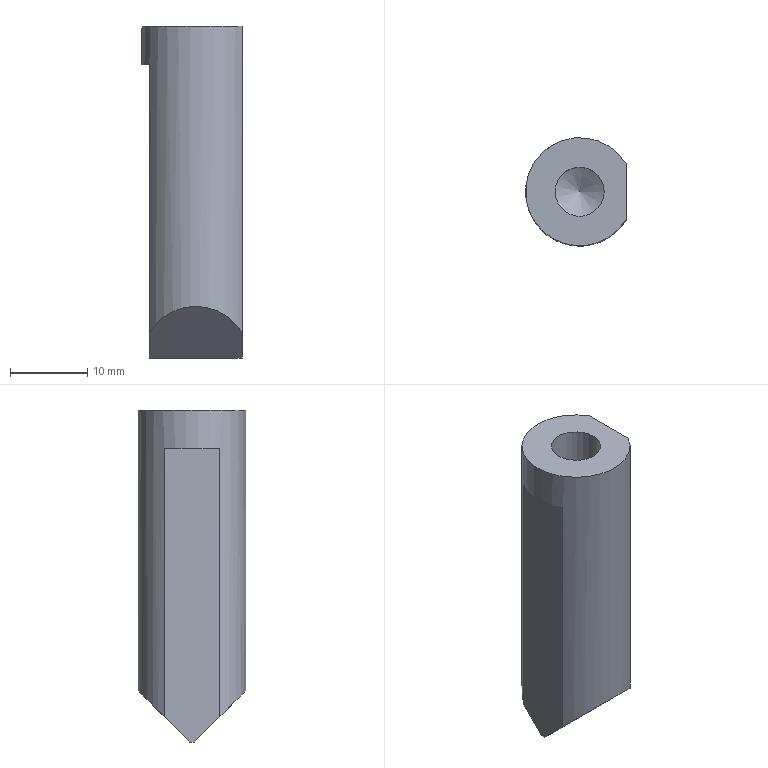Part | STEP file | 1_id278_x_t | 1 solid | 10 faces | box 13 x 14 x 43 mm | volume 5330 mm3 | plane 7 | cylinder 2 | cone 1 | commonest cylinder face diameters 6.35 x1 14 x1
STEP:
#1=CARTESIAN_POINT('',(0.,0.,0.));
#2=DIRECTION('',(0.,0.,1.));
#3=DIRECTION('',(1.,0.,0.));
#4=AXIS2_PLACEMENT_3D('',#1,#2,#3);
#5=CARTESIAN_POINT('',(759.425,181.106,-65.394));
#6=VERTEX_POINT('',#5);
#7=CARTESIAN_POINT('',(759.425,177.82,-68.68));
#8=VERTEX_POINT('',#7);
#9=CARTESIAN_POINT('',(759.425,178.5,-68.));
#10=DIRECTION('',(0.,-0.7071,-0.7071));
#11=VECTOR('',#10,1.);
#12=LINE('',#9,#11);
#13=CARTESIAN_POINT('',(771.425,178.5,-68.));
#14=DIRECTION('',(0.,-0.7071,0.7071));
#15=DIRECTION('',(0.,0.7071,0.7071));
#16=AXIS2_PLACEMENT_3D('',#13,#14,#15);
#17=PLANE('',#16);
#18=CARTESIAN_POINT('',(0.,12.));
#19=DIRECTION('',(-1.,0.));
#20=VECTOR('',#19,1.);
#21=LINE('',#18,#20);
#22=(GEOMETRIC_REPRESENTATION_CONTEXT(2)PARAMETRIC_REPRESENTATION_CONTEXT()REPRESENTATION_CONTEXT('',''));
#23=DEFINITIONAL_REPRESENTATION('',(#21),#22);
#24=PCURVE('',#17,#23);
#25=CARTESIAN_POINT('',(759.425,168.899,-15.68));
#26=DIRECTION('',(1.,0.,0.));
#27=DIRECTION('',(0.,0.,-1.));
#28=AXIS2_PLACEMENT_3D('',#25,#26,#27);
#29=PLANE('',#28);
#30=CARTESIAN_POINT('',(52.32,9.601));
#31=DIRECTION('',(0.7071,-0.7071));
#32=VECTOR('',#31,1.);
#33=LINE('',#30,#32);
#34=(GEOMETRIC_REPRESENTATION_CONTEXT(2)PARAMETRIC_REPRESENTATION_CONTEXT()REPRESENTATION_CONTEXT('',''));
#35=DEFINITIONAL_REPRESENTATION('',(#33),#34);
#36=PCURVE('',#29,#35);
#37=SURFACE_CURVE('',#12,(#24,#36),.PCURVE_S1.);
#38=EDGE_CURVE('',#6,#8,#37,.T.);
#39=ORIENTED_EDGE('',*,*,#38,.F.);
#40=CARTESIAN_POINT('',(771.425,181.106,-65.394));
#41=VERTEX_POINT('',#40);
#42=CARTESIAN_POINT('',(765.425,177.5,-69.));
#43=DIRECTION('',(0.,-0.7071,0.7071));
#44=DIRECTION('',(0.,-0.7071,-0.7071));
#45=AXIS2_PLACEMENT_3D('',#42,#43,#44);
#46=ELLIPSE('',#45,9.899,7.);
#47=CARTESIAN_POINT('',(-1.414,6.));
#48=DIRECTION('',(-1.,0.));
#49=AXIS2_PLACEMENT_2D('',#47,#48);
#50=ELLIPSE('',#49,9.899,7.);
#51=(GEOMETRIC_REPRESENTATION_CONTEXT(2)PARAMETRIC_REPRESENTATION_CONTEXT()REPRESENTATION_CONTEXT('',''));
#52=DEFINITIONAL_REPRESENTATION('',(#50),#51);
#53=PCURVE('',#17,#52);
#54=CARTESIAN_POINT('',(765.425,177.5,17.));
#55=DIRECTION('',(0.,0.,-1.));
#56=DIRECTION('',(0.,1.,0.));
#57=AXIS2_PLACEMENT_3D('',#54,#55,#56);
#58=CYLINDRICAL_SURFACE('',#57,7.);
#59=CARTESIAN_POINT('',(7.313,82.394));
#60=CARTESIAN_POINT('',(7.282,82.207));
#61=CARTESIAN_POINT('',(7.219,81.843));
#62=CARTESIAN_POINT('',(7.126,81.334));
#63=CARTESIAN_POINT('',(7.032,80.865));
#64=CARTESIAN_POINT('',(6.938,80.442));
#65=CARTESIAN_POINT('',(6.845,80.067));
#66=CARTESIAN_POINT('',(6.751,79.744));
#67=CARTESIAN_POINT('',(6.658,79.475));
#68=CARTESIAN_POINT('',(6.564,79.264));
#69=CARTESIAN_POINT('',(6.47,79.112));
#70=CARTESIAN_POINT('',(6.377,79.02));
#71=CARTESIAN_POINT('',(6.283,78.99));
#72=CARTESIAN_POINT('',(6.19,79.02));
#73=CARTESIAN_POINT('',(6.096,79.112));
#74=CARTESIAN_POINT('',(6.002,79.264));
#75=CARTESIAN_POINT('',(5.909,79.475));
#76=CARTESIAN_POINT('',(5.815,79.744));
#77=CARTESIAN_POINT('',(5.722,80.067));
#78=CARTESIAN_POINT('',(5.628,80.442));
#79=CARTESIAN_POINT('',(5.534,80.865));
#80=CARTESIAN_POINT('',(5.441,81.334));
#81=CARTESIAN_POINT('',(5.347,81.843));
#82=CARTESIAN_POINT('',(5.285,82.207));
#83=CARTESIAN_POINT('',(5.253,82.394));
#84=B_SPLINE_CURVE_WITH_KNOTS('',3,(#59,#60,#61,#62,#63,#64,#65,#66,#67,#68,#69,#70,#71,#72,#73,#74,#75,#76,#77,#78,#79,#80,#81,#82,#83),.UNSPECIFIED.,.F.,.F.,(4,1,1,1,1,1,1,1,1,1,1,1,1,1,1,1,1,1,1,1,1,1,4),(2.112,2.206,2.299,2.393,2.486,2.58,2.674,2.767,2.861,2.954,3.048,3.142,3.235,3.329,3.422,3.516,3.61,3.703,3.797,3.89,3.984,4.078,4.171),.QUASI_UNIFORM_KNOTS.);
#85=(GEOMETRIC_REPRESENTATION_CONTEXT(2)PARAMETRIC_REPRESENTATION_CONTEXT()REPRESENTATION_CONTEXT('',''));
#86=DEFINITIONAL_REPRESENTATION('',(#84),#85);
#87=PCURVE('',#58,#86);
#88=SURFACE_CURVE('',#46,(#53,#87),.PCURVE_S1.);
#89=EDGE_CURVE('',#41,#6,#88,.T.);
#90=ORIENTED_EDGE('',*,*,#89,.F.);
#91=CARTESIAN_POINT('',(771.425,177.82,-68.68));
#92=VERTEX_POINT('',#91);
#93=CARTESIAN_POINT('',(771.425,178.5,-68.));
#94=DIRECTION('',(0.,0.7071,0.7071));
#95=VECTOR('',#94,1.);
#96=LINE('',#93,#95);
#97=CARTESIAN_POINT('',(0.,0.));
#98=DIRECTION('',(1.,0.));
#99=VECTOR('',#98,1.);
#100=LINE('',#97,#99);
#101=(GEOMETRIC_REPRESENTATION_CONTEXT(2)PARAMETRIC_REPRESENTATION_CONTEXT()REPRESENTATION_CONTEXT('',''));
#102=DEFINITIONAL_REPRESENTATION('',(#100),#101);
#103=PCURVE('',#17,#102);
#104=CARTESIAN_POINT('',(771.425,170.46,30.));
#105=DIRECTION('',(1.,0.,0.));
#106=DIRECTION('',(0.,0.,1.));
#107=AXIS2_PLACEMENT_3D('',#104,#105,#106);
#108=PLANE('',#107);
#109=CARTESIAN_POINT('',(-98.,-8.04));
#110=DIRECTION('',(0.7071,-0.7071));
#111=VECTOR('',#110,1.);
#112=LINE('',#109,#111);
#113=(GEOMETRIC_REPRESENTATION_CONTEXT(2)PARAMETRIC_REPRESENTATION_CONTEXT()REPRESENTATION_CONTEXT('',''));
#114=DEFINITIONAL_REPRESENTATION('',(#112),#113);
#115=PCURVE('',#108,#114);
#116=SURFACE_CURVE('',#96,(#103,#115),.PCURVE_S1.);
#117=EDGE_CURVE('',#92,#41,#116,.T.);
#118=ORIENTED_EDGE('',*,*,#117,.F.);
#119=CARTESIAN_POINT('',(771.425,177.82,-68.68));
#120=DIRECTION('',(-1.,0.,0.));
#121=VECTOR('',#120,1.);
#122=LINE('',#119,#121);
#123=CARTESIAN_POINT('',(-0.9617,0.));
#124=DIRECTION('',(0.,1.));
#125=VECTOR('',#124,1.);
#126=LINE('',#123,#125);
#127=(GEOMETRIC_REPRESENTATION_CONTEXT(2)PARAMETRIC_REPRESENTATION_CONTEXT()REPRESENTATION_CONTEXT('',''));
#128=DEFINITIONAL_REPRESENTATION('',(#126),#127);
#129=PCURVE('',#17,#128);
#130=CARTESIAN_POINT('',(765.425,177.5,-68.68));
#131=DIRECTION('',(0.,0.,-1.));
#132=DIRECTION('',(0.,1.,0.));
#133=AXIS2_PLACEMENT_3D('',#130,#131,#132);
#134=PLANE('',#133);
#135=CARTESIAN_POINT('',(0.32,6.));
#136=DIRECTION('',(0.,-1.));
#137=VECTOR('',#136,1.);
#138=LINE('',#135,#137);
#139=(GEOMETRIC_REPRESENTATION_CONTEXT(2)PARAMETRIC_REPRESENTATION_CONTEXT()REPRESENTATION_CONTEXT('',''));
#140=DEFINITIONAL_REPRESENTATION('',(#138),#139);
#141=PCURVE('',#134,#140);
#142=SURFACE_CURVE('',#122,(#129,#141),.PCURVE_S1.);
#143=EDGE_CURVE('',#92,#8,#142,.T.);
#144=ORIENTED_EDGE('',*,*,#143,.T.);
#145=EDGE_LOOP('',(#39,#90,#118,#144));
#146=FACE_BOUND('',#145,.T.);
#147=ADVANCED_FACE('',(#146),#17,.F.);
#148=CARTESIAN_POINT('',(759.425,177.18,-68.68));
#149=VERTEX_POINT('',#148);
#150=CARTESIAN_POINT('',(759.425,177.5,-68.68));
#151=DIRECTION('',(0.,-1.,0.));
#152=VECTOR('',#151,1.);
#153=LINE('',#150,#152);
#154=CARTESIAN_POINT('',(0.,-6.));
#155=DIRECTION('',(-1.,0.));
#156=VECTOR('',#155,1.);
#157=LINE('',#154,#156);
#158=(GEOMETRIC_REPRESENTATION_CONTEXT(2)PARAMETRIC_REPRESENTATION_CONTEXT()REPRESENTATION_CONTEXT('',''));
#159=DEFINITIONAL_REPRESENTATION('',(#157),#158);
#160=PCURVE('',#134,#159);
#161=CARTESIAN_POINT('',(53.,8.601));
#162=DIRECTION('',(0.,-1.));
#163=VECTOR('',#162,1.);
#164=LINE('',#161,#163);
#165=(GEOMETRIC_REPRESENTATION_CONTEXT(2)PARAMETRIC_REPRESENTATION_CONTEXT()REPRESENTATION_CONTEXT('',''));
#166=DEFINITIONAL_REPRESENTATION('',(#164),#165);
#167=PCURVE('',#29,#166);
#168=SURFACE_CURVE('',#153,(#160,#167),.PCURVE_S1.);
#169=EDGE_CURVE('',#8,#149,#168,.T.);
#170=ORIENTED_EDGE('',*,*,#169,.F.);
#171=ORIENTED_EDGE('',*,*,#143,.F.);
#172=CARTESIAN_POINT('',(771.425,177.18,-68.68));
#173=VERTEX_POINT('',#172);
#174=CARTESIAN_POINT('',(771.425,170.46,-68.68));
#175=DIRECTION('',(0.,1.,0.));
#176=VECTOR('',#175,1.);
#177=LINE('',#174,#176);
#178=CARTESIAN_POINT('',(-7.04,6.));
#179=DIRECTION('',(1.,0.));
#180=VECTOR('',#179,1.);
#181=LINE('',#178,#180);
#182=(GEOMETRIC_REPRESENTATION_CONTEXT(2)PARAMETRIC_REPRESENTATION_CONTEXT()REPRESENTATION_CONTEXT('',''));
#183=DEFINITIONAL_REPRESENTATION('',(#181),#182);
#184=PCURVE('',#134,#183);
#185=CARTESIAN_POINT('',(-98.68,0.));
#186=DIRECTION('',(0.,-1.));
#187=VECTOR('',#186,1.);
#188=LINE('',#185,#187);
#189=(GEOMETRIC_REPRESENTATION_CONTEXT(2)PARAMETRIC_REPRESENTATION_CONTEXT()REPRESENTATION_CONTEXT('',''));
#190=DEFINITIONAL_REPRESENTATION('',(#188),#189);
#191=PCURVE('',#108,#190);
#192=SURFACE_CURVE('',#177,(#184,#191),.PCURVE_S1.);
#193=EDGE_CURVE('',#173,#92,#192,.T.);
#194=ORIENTED_EDGE('',*,*,#193,.F.);
#195=CARTESIAN_POINT('',(765.425,177.18,-68.68));
#196=DIRECTION('',(-1.,0.,0.));
#197=VECTOR('',#196,1.);
#198=LINE('',#195,#197);
#199=CARTESIAN_POINT('',(-0.32,0.));
#200=DIRECTION('',(0.,-1.));
#201=VECTOR('',#200,1.);
#202=LINE('',#199,#201);
#203=(GEOMETRIC_REPRESENTATION_CONTEXT(2)PARAMETRIC_REPRESENTATION_CONTEXT()REPRESENTATION_CONTEXT('',''));
#204=DEFINITIONAL_REPRESENTATION('',(#202),#203);
#205=PCURVE('',#134,#204);
#206=CARTESIAN_POINT('',(771.425,176.5,-68.));
#207=DIRECTION('',(0.,0.7071,0.7071));
#208=DIRECTION('',(0.,-0.7071,0.7071));
#209=AXIS2_PLACEMENT_3D('',#206,#207,#208);
#210=PLANE('',#209);
#211=CARTESIAN_POINT('',(-0.9617,-6.));
#212=DIRECTION('',(0.,-1.));
#213=VECTOR('',#212,1.);
#214=LINE('',#211,#213);
#215=(GEOMETRIC_REPRESENTATION_CONTEXT(2)PARAMETRIC_REPRESENTATION_CONTEXT()REPRESENTATION_CONTEXT('',''));
#216=DEFINITIONAL_REPRESENTATION('',(#214),#215);
#217=PCURVE('',#210,#216);
#218=SURFACE_CURVE('',#198,(#205,#217),.PCURVE_S1.);
#219=EDGE_CURVE('',#173,#149,#218,.T.);
#220=ORIENTED_EDGE('',*,*,#219,.T.);
#221=EDGE_LOOP('',(#170,#171,#194,#220));
#222=FACE_BOUND('',#221,.T.);
#223=ADVANCED_FACE('',(#222),#134,.T.);
#224=CARTESIAN_POINT('',(759.425,173.894,-65.394));
#225=VERTEX_POINT('',#224);
#226=CARTESIAN_POINT('',(759.425,176.5,-68.));
#227=DIRECTION('',(0.,-0.7071,0.7071));
#228=VECTOR('',#227,1.);
#229=LINE('',#226,#228);
#230=CARTESIAN_POINT('',(0.,-12.));
#231=DIRECTION('',(1.,0.));
#232=VECTOR('',#231,1.);
#233=LINE('',#230,#232);
#234=(GEOMETRIC_REPRESENTATION_CONTEXT(2)PARAMETRIC_REPRESENTATION_CONTEXT()REPRESENTATION_CONTEXT('',''));
#235=DEFINITIONAL_REPRESENTATION('',(#233),#234);
#236=PCURVE('',#210,#235);
#237=CARTESIAN_POINT('',(52.32,7.601));
#238=DIRECTION('',(-0.7071,-0.7071));
#239=VECTOR('',#238,1.);
#240=LINE('',#237,#239);
#241=(GEOMETRIC_REPRESENTATION_CONTEXT(2)PARAMETRIC_REPRESENTATION_CONTEXT()REPRESENTATION_CONTEXT('',''));
#242=DEFINITIONAL_REPRESENTATION('',(#240),#241);
#243=PCURVE('',#29,#242);
#244=SURFACE_CURVE('',#229,(#236,#243),.PCURVE_S1.);
#245=EDGE_CURVE('',#149,#225,#244,.T.);
#246=ORIENTED_EDGE('',*,*,#245,.F.);
#247=ORIENTED_EDGE('',*,*,#219,.F.);
#248=CARTESIAN_POINT('',(771.425,173.894,-65.394));
#249=VERTEX_POINT('',#248);
#250=CARTESIAN_POINT('',(771.425,176.5,-68.));
#251=DIRECTION('',(0.,-0.7071,0.7071));
#252=VECTOR('',#251,1.);
#253=LINE('',#250,#252);
#254=CARTESIAN_POINT('',(0.,0.));
#255=DIRECTION('',(1.,0.));
#256=VECTOR('',#255,1.);
#257=LINE('',#254,#256);
#258=(GEOMETRIC_REPRESENTATION_CONTEXT(2)PARAMETRIC_REPRESENTATION_CONTEXT()REPRESENTATION_CONTEXT('',''));
#259=DEFINITIONAL_REPRESENTATION('',(#257),#258);
#260=PCURVE('',#210,#259);
#261=CARTESIAN_POINT('',(-98.,-6.04));
#262=DIRECTION('',(0.7071,0.7071));
#263=VECTOR('',#262,1.);
#264=LINE('',#261,#263);
#265=(GEOMETRIC_REPRESENTATION_CONTEXT(2)PARAMETRIC_REPRESENTATION_CONTEXT()REPRESENTATION_CONTEXT('',''));
#266=DEFINITIONAL_REPRESENTATION('',(#264),#265);
#267=PCURVE('',#108,#266);
#268=SURFACE_CURVE('',#253,(#260,#267),.PCURVE_S1.);
#269=EDGE_CURVE('',#173,#249,#268,.T.);
#270=ORIENTED_EDGE('',*,*,#269,.T.);
#271=CARTESIAN_POINT('',(765.425,177.5,-69.));
#272=DIRECTION('',(0.,0.7071,0.7071));
#273=DIRECTION('',(0.,0.7071,-0.7071));
#274=AXIS2_PLACEMENT_3D('',#271,#272,#273);
#275=ELLIPSE('',#274,9.899,7.);
#276=CARTESIAN_POINT('',(-1.414,-6.));
#277=DIRECTION('',(-1.,0.));
#278=AXIS2_PLACEMENT_2D('',#276,#277);
#279=ELLIPSE('',#278,9.899,7.);
#280=(GEOMETRIC_REPRESENTATION_CONTEXT(2)PARAMETRIC_REPRESENTATION_CONTEXT()REPRESENTATION_CONTEXT('',''));
#281=DEFINITIONAL_REPRESENTATION('',(#279),#280);
#282=PCURVE('',#210,#281);
#283=CARTESIAN_POINT('',(4.171,82.394));
#284=CARTESIAN_POINT('',(4.14,82.207));
#285=CARTESIAN_POINT('',(4.078,81.843));
#286=CARTESIAN_POINT('',(3.984,81.334));
#287=CARTESIAN_POINT('',(3.89,80.865));
#288=CARTESIAN_POINT('',(3.797,80.442));
#289=CARTESIAN_POINT('',(3.703,80.067));
#290=CARTESIAN_POINT('',(3.61,79.744));
#291=CARTESIAN_POINT('',(3.516,79.475));
#292=CARTESIAN_POINT('',(3.422,79.264));
#293=CARTESIAN_POINT('',(3.329,79.112));
#294=CARTESIAN_POINT('',(3.235,79.02));
#295=CARTESIAN_POINT('',(3.142,78.99));
#296=CARTESIAN_POINT('',(3.048,79.02));
#297=CARTESIAN_POINT('',(2.954,79.112));
#298=CARTESIAN_POINT('',(2.861,79.264));
#299=CARTESIAN_POINT('',(2.767,79.475));
#300=CARTESIAN_POINT('',(2.674,79.744));
#301=CARTESIAN_POINT('',(2.58,80.067));
#302=CARTESIAN_POINT('',(2.486,80.442));
#303=CARTESIAN_POINT('',(2.393,80.865));
#304=CARTESIAN_POINT('',(2.299,81.334));
#305=CARTESIAN_POINT('',(2.206,81.843));
#306=CARTESIAN_POINT('',(2.143,82.207));
#307=CARTESIAN_POINT('',(2.112,82.394));
#308=B_SPLINE_CURVE_WITH_KNOTS('',3,(#283,#284,#285,#286,#287,#288,#289,#290,#291,#292,#293,#294,#295,#296,#297,#298,#299,#300,#301,#302,#303,#304,#305,#306,#307),.UNSPECIFIED.,.F.,.F.,(4,1,1,1,1,1,1,1,1,1,1,1,1,1,1,1,1,1,1,1,1,1,4),(2.112,2.206,2.299,2.393,2.486,2.58,2.674,2.767,2.861,2.954,3.048,3.142,3.235,3.329,3.422,3.516,3.61,3.703,3.797,3.89,3.984,4.078,4.171),.QUASI_UNIFORM_KNOTS.);
#309=(GEOMETRIC_REPRESENTATION_CONTEXT(2)PARAMETRIC_REPRESENTATION_CONTEXT()REPRESENTATION_CONTEXT('',''));
#310=DEFINITIONAL_REPRESENTATION('',(#308),#309);
#311=PCURVE('',#58,#310);
#312=SURFACE_CURVE('',#275,(#282,#311),.PCURVE_S1.);
#313=EDGE_CURVE('',#225,#249,#312,.T.);
#314=ORIENTED_EDGE('',*,*,#313,.F.);
#315=EDGE_LOOP('',(#246,#247,#270,#314));
#316=FACE_BOUND('',#315,.T.);
#317=ADVANCED_FACE('',(#316),#210,.F.);
#318=CARTESIAN_POINT('',(771.425,181.106,-25.68));
#319=VERTEX_POINT('',#318);
#320=CARTESIAN_POINT('',(771.425,181.106,17.));
#321=DIRECTION('',(0.,0.,-1.));
#322=VECTOR('',#321,1.);
#323=LINE('',#320,#322);
#324=CARTESIAN_POINT('',(-13.,-10.645));
#325=DIRECTION('',(-1.,0.));
#326=VECTOR('',#325,1.);
#327=LINE('',#324,#326);
#328=(GEOMETRIC_REPRESENTATION_CONTEXT(2)PARAMETRIC_REPRESENTATION_CONTEXT()REPRESENTATION_CONTEXT('',''));
#329=DEFINITIONAL_REPRESENTATION('',(#327),#328);
#330=PCURVE('',#108,#329);
#331=CARTESIAN_POINT('',(7.313,0.));
#332=DIRECTION('',(0.,1.));
#333=VECTOR('',#332,1.);
#334=LINE('',#331,#333);
#335=(GEOMETRIC_REPRESENTATION_CONTEXT(2)PARAMETRIC_REPRESENTATION_CONTEXT()REPRESENTATION_CONTEXT('',''));
#336=DEFINITIONAL_REPRESENTATION('',(#334),#335);
#337=PCURVE('',#58,#336);
#338=SURFACE_CURVE('',#323,(#330,#337),.PCURVE_S1.);
#339=EDGE_CURVE('',#319,#41,#338,.T.);
#340=ORIENTED_EDGE('',*,*,#339,.F.);
#341=CARTESIAN_POINT('',(771.425,173.894,-25.68));
#342=VERTEX_POINT('',#341);
#343=CARTESIAN_POINT('',(771.425,177.5,-25.68));
#344=DIRECTION('',(0.,-1.,0.));
#345=VECTOR('',#344,1.);
#346=LINE('',#343,#345);
#347=CARTESIAN_POINT('',(-55.68,-7.04));
#348=DIRECTION('',(0.,1.));
#349=VECTOR('',#348,1.);
#350=LINE('',#347,#349);
#351=(GEOMETRIC_REPRESENTATION_CONTEXT(2)PARAMETRIC_REPRESENTATION_CONTEXT()REPRESENTATION_CONTEXT('',''));
#352=DEFINITIONAL_REPRESENTATION('',(#350),#351);
#353=PCURVE('',#108,#352);
#354=CARTESIAN_POINT('',(780.775,177.5,-25.68));
#355=DIRECTION('',(0.,0.,-1.));
#356=DIRECTION('',(0.,1.,0.));
#357=AXIS2_PLACEMENT_3D('',#354,#355,#356);
#358=PLANE('',#357);
#359=CARTESIAN_POINT('',(0.,-9.35));
#360=DIRECTION('',(-1.,0.));
#361=VECTOR('',#360,1.);
#362=LINE('',#359,#361);
#363=(GEOMETRIC_REPRESENTATION_CONTEXT(2)PARAMETRIC_REPRESENTATION_CONTEXT()REPRESENTATION_CONTEXT('',''));
#364=DEFINITIONAL_REPRESENTATION('',(#362),#363);
#365=PCURVE('',#358,#364);
#366=SURFACE_CURVE('',#346,(#353,#365),.PCURVE_S1.);
#367=EDGE_CURVE('',#319,#342,#366,.T.);
#368=ORIENTED_EDGE('',*,*,#367,.T.);
#369=CARTESIAN_POINT('',(771.425,173.894,17.));
#370=DIRECTION('',(0.,0.,1.));
#371=VECTOR('',#370,1.);
#372=LINE('',#369,#371);
#373=CARTESIAN_POINT('',(-13.,-3.434));
#374=DIRECTION('',(1.,0.));
#375=VECTOR('',#374,1.);
#376=LINE('',#373,#375);
#377=(GEOMETRIC_REPRESENTATION_CONTEXT(2)PARAMETRIC_REPRESENTATION_CONTEXT()REPRESENTATION_CONTEXT('',''));
#378=DEFINITIONAL_REPRESENTATION('',(#376),#377);
#379=PCURVE('',#108,#378);
#380=CARTESIAN_POINT('',(2.112,0.));
#381=DIRECTION('',(0.,-1.));
#382=VECTOR('',#381,1.);
#383=LINE('',#380,#382);
#384=(GEOMETRIC_REPRESENTATION_CONTEXT(2)PARAMETRIC_REPRESENTATION_CONTEXT()REPRESENTATION_CONTEXT('',''));
#385=DEFINITIONAL_REPRESENTATION('',(#383),#384);
#386=PCURVE('',#58,#385);
#387=SURFACE_CURVE('',#372,(#379,#386),.PCURVE_S1.);
#388=EDGE_CURVE('',#249,#342,#387,.T.);
#389=ORIENTED_EDGE('',*,*,#388,.F.);
#390=ORIENTED_EDGE('',*,*,#269,.F.);
#391=ORIENTED_EDGE('',*,*,#193,.T.);
#392=ORIENTED_EDGE('',*,*,#117,.T.);
#393=EDGE_LOOP('',(#340,#368,#389,#390,#391,#392));
#394=FACE_BOUND('',#393,.T.);
#395=ADVANCED_FACE('',(#394),#108,.T.);
#396=CARTESIAN_POINT('',(759.425,181.106,-30.68));
#397=VERTEX_POINT('',#396);
#398=CARTESIAN_POINT('',(759.425,181.106,17.));
#399=DIRECTION('',(0.,0.,-1.));
#400=VECTOR('',#399,1.);
#401=LINE('',#398,#400);
#402=CARTESIAN_POINT('',(5.253,0.));
#403=DIRECTION('',(0.,1.));
#404=VECTOR('',#403,1.);
#405=LINE('',#402,#404);
#406=(GEOMETRIC_REPRESENTATION_CONTEXT(2)PARAMETRIC_REPRESENTATION_CONTEXT()REPRESENTATION_CONTEXT('',''));
#407=DEFINITIONAL_REPRESENTATION('',(#405),#406);
#408=PCURVE('',#58,#407);
#409=CARTESIAN_POINT('',(-32.68,12.206));
#410=DIRECTION('',(1.,0.));
#411=VECTOR('',#410,1.);
#412=LINE('',#409,#411);
#413=(GEOMETRIC_REPRESENTATION_CONTEXT(2)PARAMETRIC_REPRESENTATION_CONTEXT()REPRESENTATION_CONTEXT('',''));
#414=DEFINITIONAL_REPRESENTATION('',(#412),#413);
#415=PCURVE('',#29,#414);
#416=SURFACE_CURVE('',#401,(#408,#415),.PCURVE_S1.);
#417=EDGE_CURVE('',#397,#6,#416,.T.);
#418=ORIENTED_EDGE('',*,*,#417,.F.);
#419=CARTESIAN_POINT('',(759.425,173.894,-30.68));
#420=VERTEX_POINT('',#419);
#421=CARTESIAN_POINT('',(765.425,177.5,-30.68));
#422=DIRECTION('',(0.,0.,-1.));
#423=DIRECTION('',(-1.,0.,0.));
#424=AXIS2_PLACEMENT_3D('',#421,#422,#423);
#425=CIRCLE('',#424,7.);
#426=CARTESIAN_POINT('',(-1.571,47.68));
#427=DIRECTION('',(1.,0.));
#428=VECTOR('',#427,1.);
#429=LINE('',#426,#428);
#430=(GEOMETRIC_REPRESENTATION_CONTEXT(2)PARAMETRIC_REPRESENTATION_CONTEXT()REPRESENTATION_CONTEXT('',''));
#431=DEFINITIONAL_REPRESENTATION('',(#429),#430);
#432=PCURVE('',#58,#431);
#433=CARTESIAN_POINT('',(764.925,177.5,-30.68));
#434=DIRECTION('',(0.,0.,1.));
#435=DIRECTION('',(-1.,0.,0.));
#436=AXIS2_PLACEMENT_3D('',#433,#434,#435);
#437=PLANE('',#436);
#438=CARTESIAN_POINT('',(6.5,0.));
#439=CARTESIAN_POINT('',(6.5,-12.124));
#440=CARTESIAN_POINT('',(-4.,-6.062));
#441=CARTESIAN_POINT('',(-14.5,0.));
#442=CARTESIAN_POINT('',(-4.,6.062));
#443=CARTESIAN_POINT('',(6.5,12.124));
#444=CARTESIAN_POINT('',(6.5,0.));
#445=(BOUNDED_CURVE()B_SPLINE_CURVE(2,(#438,#439,#440,#441,#442,#443,#444),.UNSPECIFIED.,.T.,.F.)B_SPLINE_CURVE_WITH_KNOTS((1,2,2,2,2,1),(-2.094,0.,2.094,4.189,6.283,8.378),.UNSPECIFIED.)CURVE()GEOMETRIC_REPRESENTATION_ITEM()RATIONAL_B_SPLINE_CURVE((1.,0.5,1.,0.5,1.,0.5,1.))REPRESENTATION_ITEM(''));
#446=(GEOMETRIC_REPRESENTATION_CONTEXT(2)PARAMETRIC_REPRESENTATION_CONTEXT()REPRESENTATION_CONTEXT('',''));
#447=DEFINITIONAL_REPRESENTATION('',(#445),#446);
#448=PCURVE('',#437,#447);
#449=SURFACE_CURVE('',#425,(#432,#448),.PCURVE_S1.);
#450=EDGE_CURVE('',#420,#397,#449,.T.);
#451=ORIENTED_EDGE('',*,*,#450,.F.);
#452=CARTESIAN_POINT('',(759.425,173.894,17.));
#453=DIRECTION('',(0.,0.,1.));
#454=VECTOR('',#453,1.);
#455=LINE('',#452,#454);
#456=CARTESIAN_POINT('',(4.171,0.));
#457=DIRECTION('',(0.,-1.));
#458=VECTOR('',#457,1.);
#459=LINE('',#456,#458);
#460=(GEOMETRIC_REPRESENTATION_CONTEXT(2)PARAMETRIC_REPRESENTATION_CONTEXT()REPRESENTATION_CONTEXT('',''));
#461=DEFINITIONAL_REPRESENTATION('',(#459),#460);
#462=PCURVE('',#58,#461);
#463=CARTESIAN_POINT('',(-32.68,4.995));
#464=DIRECTION('',(-1.,0.));
#465=VECTOR('',#464,1.);
#466=LINE('',#463,#465);
#467=(GEOMETRIC_REPRESENTATION_CONTEXT(2)PARAMETRIC_REPRESENTATION_CONTEXT()REPRESENTATION_CONTEXT('',''));
#468=DEFINITIONAL_REPRESENTATION('',(#466),#467);
#469=PCURVE('',#29,#468);
#470=SURFACE_CURVE('',#455,(#462,#469),.PCURVE_S1.);
#471=EDGE_CURVE('',#225,#420,#470,.T.);
#472=ORIENTED_EDGE('',*,*,#471,.F.);
#473=ORIENTED_EDGE('',*,*,#313,.T.);
#474=ORIENTED_EDGE('',*,*,#388,.T.);
#475=CARTESIAN_POINT('',(765.425,177.5,-25.68));
#476=DIRECTION('',(0.,0.,-1.));
#477=DIRECTION('',(1.,0.,0.));
#478=AXIS2_PLACEMENT_3D('',#475,#476,#477);
#479=CIRCLE('',#478,7.);
#480=CARTESIAN_POINT('',(1.571,42.68));
#481=DIRECTION('',(1.,0.));
#482=VECTOR('',#481,1.);
#483=LINE('',#480,#482);
#484=(GEOMETRIC_REPRESENTATION_CONTEXT(2)PARAMETRIC_REPRESENTATION_CONTEXT()REPRESENTATION_CONTEXT('',''));
#485=DEFINITIONAL_REPRESENTATION('',(#483),#484);
#486=PCURVE('',#58,#485);
#487=CARTESIAN_POINT('',(0.,-15.35));
#488=DIRECTION('',(0.,1.));
#489=AXIS2_PLACEMENT_2D('',#487,#488);
#490=CIRCLE('',#489,7.);
#491=(GEOMETRIC_REPRESENTATION_CONTEXT(2)PARAMETRIC_REPRESENTATION_CONTEXT()REPRESENTATION_CONTEXT('',''));
#492=DEFINITIONAL_REPRESENTATION('',(#490),#491);
#493=PCURVE('',#358,#492);
#494=SURFACE_CURVE('',#479,(#486,#493),.PCURVE_S1.);
#495=EDGE_CURVE('',#342,#319,#494,.T.);
#496=ORIENTED_EDGE('',*,*,#495,.T.);
#497=ORIENTED_EDGE('',*,*,#339,.T.);
#498=ORIENTED_EDGE('',*,*,#89,.T.);
#499=EDGE_LOOP('',(#418,#451,#472,#473,#474,#496,#497,#498));
#500=FACE_BOUND('',#499,.T.);
#501=ADVANCED_FACE('',(#500),#58,.T.);
#502=ORIENTED_EDGE('',*,*,#169,.T.);
#503=ORIENTED_EDGE('',*,*,#245,.T.);
#504=ORIENTED_EDGE('',*,*,#471,.T.);
#505=CARTESIAN_POINT('',(759.425,177.5,-30.68));
#506=DIRECTION('',(0.,1.,0.));
#507=VECTOR('',#506,1.);
#508=LINE('',#505,#507);
#509=CARTESIAN_POINT('',(15.,8.601));
#510=DIRECTION('',(0.,1.));
#511=VECTOR('',#510,1.);
#512=LINE('',#509,#511);
#513=(GEOMETRIC_REPRESENTATION_CONTEXT(2)PARAMETRIC_REPRESENTATION_CONTEXT()REPRESENTATION_CONTEXT('',''));
#514=DEFINITIONAL_REPRESENTATION('',(#512),#513);
#515=PCURVE('',#29,#514);
#516=CARTESIAN_POINT('',(5.5,0.));
#517=DIRECTION('',(0.,-1.));
#518=VECTOR('',#517,1.);
#519=LINE('',#516,#518);
#520=(GEOMETRIC_REPRESENTATION_CONTEXT(2)PARAMETRIC_REPRESENTATION_CONTEXT()REPRESENTATION_CONTEXT('',''));
#521=DEFINITIONAL_REPRESENTATION('',(#519),#520);
#522=PCURVE('',#437,#521);
#523=SURFACE_CURVE('',#508,(#515,#522),.PCURVE_S1.);
#524=EDGE_CURVE('',#420,#397,#523,.T.);
#525=ORIENTED_EDGE('',*,*,#524,.T.);
#526=ORIENTED_EDGE('',*,*,#417,.T.);
#527=ORIENTED_EDGE('',*,*,#38,.T.);
#528=EDGE_LOOP('',(#502,#503,#504,#525,#526,#527));
#529=FACE_BOUND('',#528,.T.);
#530=ADVANCED_FACE('',(#529),#29,.F.);
#531=CARTESIAN_POINT('',(762.25,177.5,-25.68));
#532=VERTEX_POINT('',#531);
#533=CARTESIAN_POINT('',(765.425,177.5,-25.68));
#534=DIRECTION('',(0.,0.,-1.));
#535=DIRECTION('',(-1.,0.,0.));
#536=AXIS2_PLACEMENT_3D('',#533,#534,#535);
#537=CIRCLE('',#536,3.175);
#538=CARTESIAN_POINT('',(0.,-15.35));
#539=DIRECTION('',(0.,-1.));
#540=AXIS2_PLACEMENT_2D('',#538,#539);
#541=CIRCLE('',#540,3.175);
#542=(GEOMETRIC_REPRESENTATION_CONTEXT(2)PARAMETRIC_REPRESENTATION_CONTEXT()REPRESENTATION_CONTEXT('',''));
#543=DEFINITIONAL_REPRESENTATION('',(#541),#542);
#544=PCURVE('',#358,#543);
#545=CARTESIAN_POINT('',(765.425,177.5,-25.68));
#546=DIRECTION('',(0.,0.,-1.));
#547=DIRECTION('',(-1.,0.,0.));
#548=AXIS2_PLACEMENT_3D('',#545,#546,#547);
#549=CYLINDRICAL_SURFACE('',#548,3.175);
#550=CARTESIAN_POINT('',(0.,0.));
#551=DIRECTION('',(1.,0.));
#552=VECTOR('',#551,1.);
#553=LINE('',#550,#552);
#554=(GEOMETRIC_REPRESENTATION_CONTEXT(2)PARAMETRIC_REPRESENTATION_CONTEXT()REPRESENTATION_CONTEXT('',''));
#555=DEFINITIONAL_REPRESENTATION('',(#553),#554);
#556=PCURVE('',#549,#555);
#557=SURFACE_CURVE('',#537,(#544,#556),.PCURVE_S1.);
#558=EDGE_CURVE('',#532,#532,#557,.T.);
#559=ORIENTED_EDGE('',*,*,#558,.T.);
#560=EDGE_LOOP('',(#559));
#561=FACE_BOUND('',#560,.T.);
#562=ORIENTED_EDGE('',*,*,#367,.F.);
#563=ORIENTED_EDGE('',*,*,#495,.F.);
#564=EDGE_LOOP('',(#562,#563));
#565=FACE_BOUND('',#564,.T.);
#566=ADVANCED_FACE('',(#561,#565),#358,.F.);
#567=ORIENTED_EDGE('',*,*,#524,.F.);
#568=ORIENTED_EDGE('',*,*,#450,.T.);
#569=EDGE_LOOP('',(#567,#568));
#570=FACE_BOUND('',#569,.T.);
#571=ADVANCED_FACE('',(#570),#437,.F.);
#572=CARTESIAN_POINT('',(762.25,177.5,-40.68));
#573=VERTEX_POINT('',#572);
#574=CARTESIAN_POINT('',(768.6,177.5,-40.68));
#575=VERTEX_POINT('',#574);
#576=CARTESIAN_POINT('',(765.425,177.5,-40.68));
#577=DIRECTION('',(0.,0.,-1.));
#578=DIRECTION('',(-1.,0.,0.));
#579=AXIS2_PLACEMENT_3D('',#576,#577,#578);
#580=CIRCLE('',#579,3.175);
#581=CARTESIAN_POINT('',(765.425,177.5,-40.68));
#582=DIRECTION('',(0.,0.,1.));
#583=DIRECTION('',(1.,0.,0.));
#584=AXIS2_PLACEMENT_3D('',#581,#582,#583);
#585=CONICAL_SURFACE('',#584,3.175,1.03);
#586=CARTESIAN_POINT('',(3.142,0.));
#587=DIRECTION('',(-1.,0.));
#588=VECTOR('',#587,1.);
#589=LINE('',#586,#588);
#590=(GEOMETRIC_REPRESENTATION_CONTEXT(2)PARAMETRIC_REPRESENTATION_CONTEXT()REPRESENTATION_CONTEXT('',''));
#591=DEFINITIONAL_REPRESENTATION('',(#589),#590);
#592=PCURVE('',#585,#591);
#593=CARTESIAN_POINT('',(0.,15.));
#594=DIRECTION('',(1.,0.));
#595=VECTOR('',#594,1.);
#596=LINE('',#593,#595);
#597=(GEOMETRIC_REPRESENTATION_CONTEXT(2)PARAMETRIC_REPRESENTATION_CONTEXT()REPRESENTATION_CONTEXT('',''));
#598=DEFINITIONAL_REPRESENTATION('',(#596),#597);
#599=PCURVE('',#549,#598);
#600=SURFACE_CURVE('',#580,(#592,#599),.PCURVE_S1.);
#601=EDGE_CURVE('',#573,#575,#600,.T.);
#602=ORIENTED_EDGE('',*,*,#601,.T.);
#603=CARTESIAN_POINT('',(765.425,177.5,-42.588));
#604=VERTEX_POINT('',#603);
#605=CARTESIAN_POINT('',(765.425,177.5,-42.588));
#606=CARTESIAN_POINT('',(768.6,177.5,-40.68));
#607=B_SPLINE_CURVE_WITH_KNOTS('',1,(#605,#606),.UNSPECIFIED.,.F.,.F.,(2,2),(-3.704,0.),.PIECEWISE_BEZIER_KNOTS.);
#608=CARTESIAN_POINT('',(0.,0.));
#609=DIRECTION('',(0.,1.));
#610=VECTOR('',#609,1.);
#611=LINE('',#608,#610);
#612=(GEOMETRIC_REPRESENTATION_CONTEXT(2)PARAMETRIC_REPRESENTATION_CONTEXT()REPRESENTATION_CONTEXT('',''));
#613=DEFINITIONAL_REPRESENTATION('',(#611),#612);
#614=PCURVE('',#585,#613);
#615=CARTESIAN_POINT('',(6.283,0.));
#616=DIRECTION('',(0.,1.));
#617=VECTOR('',#616,1.);
#618=LINE('',#615,#617);
#619=(GEOMETRIC_REPRESENTATION_CONTEXT(2)PARAMETRIC_REPRESENTATION_CONTEXT()REPRESENTATION_CONTEXT('',''));
#620=DEFINITIONAL_REPRESENTATION('',(#618),#619);
#621=PCURVE('',#585,#620);
#622=SEAM_CURVE('',#607,(#614,#621),.PCURVE_S1.);
#623=EDGE_CURVE('',#604,#575,#622,.T.);
#624=ORIENTED_EDGE('',*,*,#623,.F.);
#625=ORIENTED_EDGE('',*,*,#623,.T.);
#626=CARTESIAN_POINT('',(765.425,177.5,-40.68));
#627=DIRECTION('',(0.,0.,-1.));
#628=DIRECTION('',(-1.,0.,0.));
#629=AXIS2_PLACEMENT_3D('',#626,#627,#628);
#630=CIRCLE('',#629,3.175);
#631=CARTESIAN_POINT('',(9.425,0.));
#632=DIRECTION('',(-1.,0.));
#633=VECTOR('',#632,1.);
#634=LINE('',#631,#633);
#635=(GEOMETRIC_REPRESENTATION_CONTEXT(2)PARAMETRIC_REPRESENTATION_CONTEXT()REPRESENTATION_CONTEXT('',''));
#636=DEFINITIONAL_REPRESENTATION('',(#634),#635);
#637=PCURVE('',#585,#636);
#638=CARTESIAN_POINT('',(0.,15.));
#639=DIRECTION('',(1.,0.));
#640=VECTOR('',#639,1.);
#641=LINE('',#638,#640);
#642=(GEOMETRIC_REPRESENTATION_CONTEXT(2)PARAMETRIC_REPRESENTATION_CONTEXT()REPRESENTATION_CONTEXT('',''));
#643=DEFINITIONAL_REPRESENTATION('',(#641),#642);
#644=PCURVE('',#549,#643);
#645=SURFACE_CURVE('',#630,(#637,#644),.PCURVE_S1.);
#646=EDGE_CURVE('',#575,#573,#645,.T.);
#647=ORIENTED_EDGE('',*,*,#646,.T.);
#648=EDGE_LOOP('',(#602,#624,#625,#647));
#649=FACE_BOUND('',#648,.F.);
#650=ADVANCED_FACE('',(#649),#585,.F.);
#651=ORIENTED_EDGE('',*,*,#646,.F.);
#652=ORIENTED_EDGE('',*,*,#601,.F.);
#653=CARTESIAN_POINT('',(762.25,177.5,-25.68));
#654=CARTESIAN_POINT('',(762.25,177.5,-40.68));
#655=B_SPLINE_CURVE_WITH_KNOTS('',1,(#653,#654),.UNSPECIFIED.,.F.,.F.,(2,2),(0.,15.),.PIECEWISE_BEZIER_KNOTS.);
#656=CARTESIAN_POINT('',(0.,0.));
#657=DIRECTION('',(0.,1.));
#658=VECTOR('',#657,1.);
#659=LINE('',#656,#658);
#660=(GEOMETRIC_REPRESENTATION_CONTEXT(2)PARAMETRIC_REPRESENTATION_CONTEXT()REPRESENTATION_CONTEXT('',''));
#661=DEFINITIONAL_REPRESENTATION('',(#659),#660);
#662=PCURVE('',#549,#661);
#663=CARTESIAN_POINT('',(6.283,0.));
#664=DIRECTION('',(0.,1.));
#665=VECTOR('',#664,1.);
#666=LINE('',#663,#665);
#667=(GEOMETRIC_REPRESENTATION_CONTEXT(2)PARAMETRIC_REPRESENTATION_CONTEXT()REPRESENTATION_CONTEXT('',''));
#668=DEFINITIONAL_REPRESENTATION('',(#666),#667);
#669=PCURVE('',#549,#668);
#670=SEAM_CURVE('',#655,(#662,#669),.PCURVE_S1.);
#671=EDGE_CURVE('',#532,#573,#670,.T.);
#672=ORIENTED_EDGE('',*,*,#671,.F.);
#673=ORIENTED_EDGE('',*,*,#558,.T.);
#674=ORIENTED_EDGE('',*,*,#671,.T.);
#675=EDGE_LOOP('',(#651,#652,#672,#673,#674));
#676=FACE_BOUND('',#675,.F.);
#677=ADVANCED_FACE('',(#676),#549,.F.);
#678=CLOSED_SHELL('',(#147,#223,#317,#395,#501,#530,#566,#571,#650,#677));
#679=MANIFOLD_SOLID_BREP('',#678);
#680=(LENGTH_UNIT()NAMED_UNIT(*)SI_UNIT(.MILLI.,.METRE.));
#681=UNCERTAINTY_MEASURE_WITH_UNIT(LENGTH_MEASURE(0.000002),#680,'','');
#682=(NAMED_UNIT(*)PLANE_ANGLE_UNIT()SI_UNIT($,.RADIAN.));
#683=(NAMED_UNIT(*)SI_UNIT($,.STERADIAN.)SOLID_ANGLE_UNIT());
#684=(GEOMETRIC_REPRESENTATION_CONTEXT(3)GLOBAL_UNCERTAINTY_ASSIGNED_CONTEXT((#681))GLOBAL_UNIT_ASSIGNED_CONTEXT((#680,#682,#683))REPRESENTATION_CONTEXT('',''));
#685=ADVANCED_BREP_SHAPE_REPRESENTATION('',(#4,#679),#684);